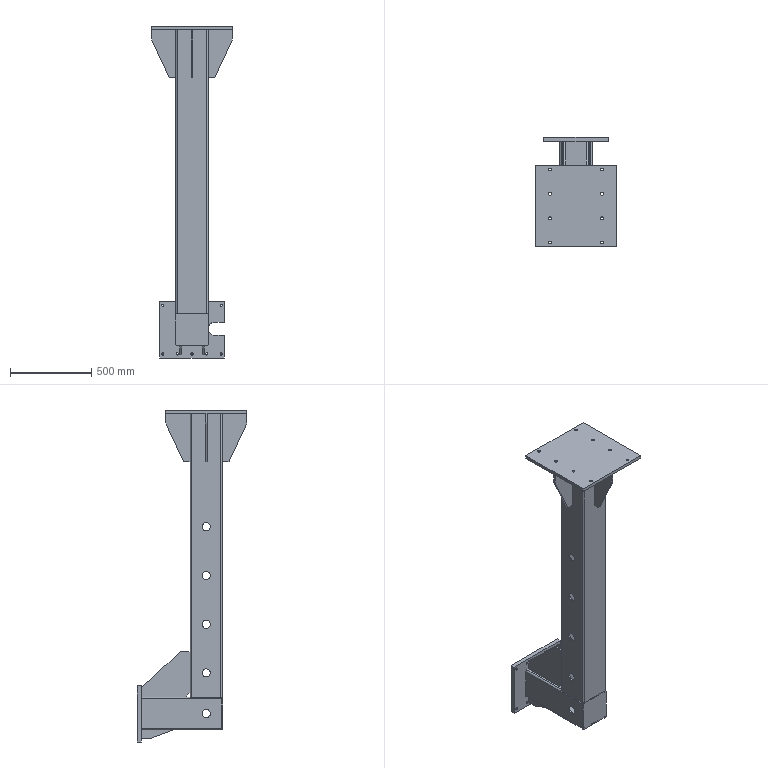Part | STEP file | YCD14007A-08.01.03 Column | 3 solids | 172 faces | box 500 x 676 x 2044 mm | volume 25161780 mm3 | plane 87 | cylinder 85 | commonest cylinder face diameters 14 x22 20 x22 50 x20 17.5 x16 1 x2 16 x2